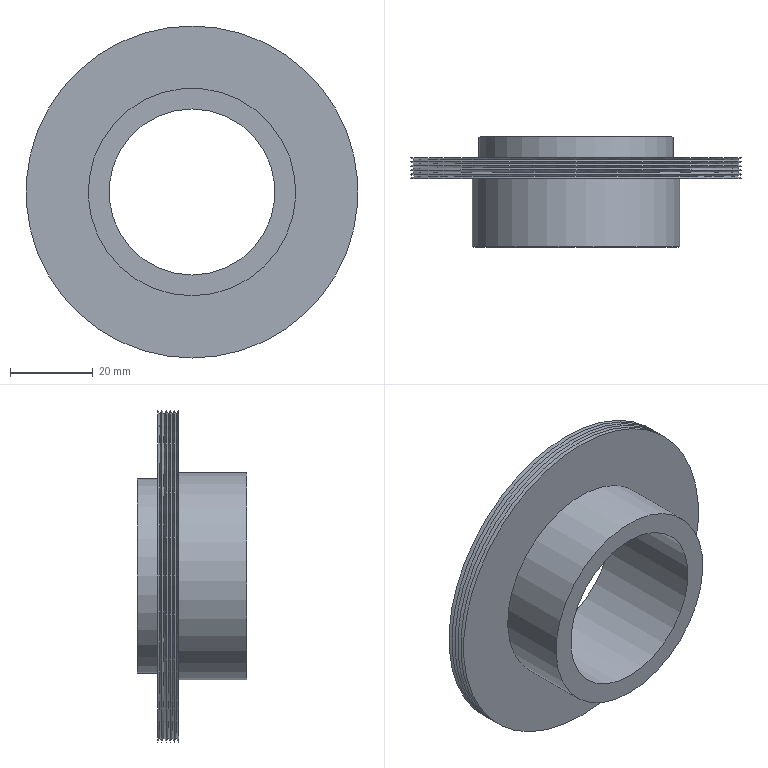Part | NX | 1 solid | 17 faces | box 80 x 26.5 x 80 mm | volume 32281 mm3 | cone 10 | plane 4 | cylinder 3 | commonest cylinder face diameters 40 x1 47 x1 50 x1
STEP:
#1=CARTESIAN_POINT('',(0.,25.732,-40.));
#2=VERTEX_POINT('',#1);
#3=CARTESIAN_POINT('',(0.,25.732,0.));
#4=DIRECTION('',(0.,-1.,0.));
#5=DIRECTION('',(0.,0.,-1.));
#6=AXIS2_PLACEMENT_3D('',#3,#4,#5);
#7=CIRCLE('',#6,40.);
#8=EDGE_CURVE('',#2,#2,#7,.T.);
#9=ORIENTED_EDGE('',*,*,#8,.F.);
#10=EDGE_LOOP('',(#9));
#11=FACE_BOUND('',#10,.T.);
#12=CARTESIAN_POINT('',(0.,25.732,-23.5));
#13=VERTEX_POINT('',#12);
#14=CARTESIAN_POINT('',(0.,25.732,0.));
#15=DIRECTION('',(0.,-1.,0.));
#16=DIRECTION('',(0.,0.,-1.));
#17=AXIS2_PLACEMENT_3D('',#14,#15,#16);
#18=CIRCLE('',#17,23.5);
#19=EDGE_CURVE('',#13,#13,#18,.T.);
#20=ORIENTED_EDGE('',*,*,#19,.T.);
#21=EDGE_LOOP('',(#20));
#22=FACE_BOUND('',#21,.T.);
#23=CARTESIAN_POINT('',(23.5,25.732,0.));
#24=DIRECTION('',(0.,-1.,0.));
#25=DIRECTION('',(0.,0.,1.));
#26=AXIS2_PLACEMENT_3D('',#23,#24,#25);
#27=PLANE('',#26);
#28=ADVANCED_FACE('',(#11,#22),#27,.F.);
#29=CARTESIAN_POINT('',(0.,25.232,-39.));
#30=VERTEX_POINT('',#29);
#31=CARTESIAN_POINT('',(0.,25.232,0.));
#32=DIRECTION('',(0.,-1.,0.));
#33=DIRECTION('',(0.,0.,-1.));
#34=AXIS2_PLACEMENT_3D('',#31,#32,#33);
#35=CIRCLE('',#34,39.);
#36=EDGE_CURVE('',#30,#30,#35,.T.);
#37=ORIENTED_EDGE('',*,*,#36,.F.);
#38=EDGE_LOOP('',(#37));
#39=FACE_BOUND('',#38,.T.);
#40=ORIENTED_EDGE('',*,*,#8,.T.);
#41=EDGE_LOOP('',(#40));
#42=FACE_BOUND('',#41,.T.);
#43=CARTESIAN_POINT('',(0.,25.732,0.));
#44=DIRECTION('',(0.,1.,0.));
#45=DIRECTION('',(0.,0.,-1.));
#46=AXIS2_PLACEMENT_3D('',#43,#44,#45);
#47=CONICAL_SURFACE('',#46,40.,63.435);
#48=ADVANCED_FACE('',(#39,#42),#47,.T.);
#49=CARTESIAN_POINT('',(0.,24.732,-40.));
#50=VERTEX_POINT('',#49);
#51=CARTESIAN_POINT('',(0.,24.732,0.));
#52=DIRECTION('',(0.,-1.,0.));
#53=DIRECTION('',(0.,0.,-1.));
#54=AXIS2_PLACEMENT_3D('',#51,#52,#53);
#55=CIRCLE('',#54,40.);
#56=EDGE_CURVE('',#50,#50,#55,.T.);
#57=ORIENTED_EDGE('',*,*,#56,.F.);
#58=EDGE_LOOP('',(#57));
#59=FACE_BOUND('',#58,.T.);
#60=ORIENTED_EDGE('',*,*,#36,.T.);
#61=EDGE_LOOP('',(#60));
#62=FACE_BOUND('',#61,.T.);
#63=CARTESIAN_POINT('',(0.,25.232,0.));
#64=DIRECTION('',(0.,-1.,0.));
#65=DIRECTION('',(0.,0.,1.));
#66=AXIS2_PLACEMENT_3D('',#63,#64,#65);
#67=CONICAL_SURFACE('',#66,39.,63.435);
#68=ADVANCED_FACE('',(#59,#62),#67,.T.);
#69=CARTESIAN_POINT('',(0.,24.232,-39.));
#70=VERTEX_POINT('',#69);
#71=CARTESIAN_POINT('',(0.,24.232,0.));
#72=DIRECTION('',(0.,-1.,0.));
#73=DIRECTION('',(0.,0.,-1.));
#74=AXIS2_PLACEMENT_3D('',#71,#72,#73);
#75=CIRCLE('',#74,39.);
#76=EDGE_CURVE('',#70,#70,#75,.T.);
#77=ORIENTED_EDGE('',*,*,#76,.F.);
#78=EDGE_LOOP('',(#77));
#79=FACE_BOUND('',#78,.T.);
#80=ORIENTED_EDGE('',*,*,#56,.T.);
#81=EDGE_LOOP('',(#80));
#82=FACE_BOUND('',#81,.T.);
#83=CARTESIAN_POINT('',(0.,24.732,0.));
#84=DIRECTION('',(0.,1.,0.));
#85=DIRECTION('',(0.,0.,-1.));
#86=AXIS2_PLACEMENT_3D('',#83,#84,#85);
#87=CONICAL_SURFACE('',#86,40.,63.435);
#88=ADVANCED_FACE('',(#79,#82),#87,.T.);
#89=CARTESIAN_POINT('',(0.,23.732,-40.));
#90=VERTEX_POINT('',#89);
#91=CARTESIAN_POINT('',(0.,23.732,0.));
#92=DIRECTION('',(0.,-1.,0.));
#93=DIRECTION('',(0.,0.,-1.));
#94=AXIS2_PLACEMENT_3D('',#91,#92,#93);
#95=CIRCLE('',#94,40.);
#96=EDGE_CURVE('',#90,#90,#95,.T.);
#97=ORIENTED_EDGE('',*,*,#96,.F.);
#98=EDGE_LOOP('',(#97));
#99=FACE_BOUND('',#98,.T.);
#100=ORIENTED_EDGE('',*,*,#76,.T.);
#101=EDGE_LOOP('',(#100));
#102=FACE_BOUND('',#101,.T.);
#103=CARTESIAN_POINT('',(0.,24.232,0.));
#104=DIRECTION('',(0.,-1.,0.));
#105=DIRECTION('',(0.,0.,1.));
#106=AXIS2_PLACEMENT_3D('',#103,#104,#105);
#107=CONICAL_SURFACE('',#106,39.,63.435);
#108=ADVANCED_FACE('',(#99,#102),#107,.T.);
#109=CARTESIAN_POINT('',(0.,23.232,-39.));
#110=VERTEX_POINT('',#109);
#111=CARTESIAN_POINT('',(0.,23.232,0.));
#112=DIRECTION('',(0.,-1.,0.));
#113=DIRECTION('',(0.,0.,-1.));
#114=AXIS2_PLACEMENT_3D('',#111,#112,#113);
#115=CIRCLE('',#114,39.);
#116=EDGE_CURVE('',#110,#110,#115,.T.);
#117=ORIENTED_EDGE('',*,*,#116,.F.);
#118=EDGE_LOOP('',(#117));
#119=FACE_BOUND('',#118,.T.);
#120=ORIENTED_EDGE('',*,*,#96,.T.);
#121=EDGE_LOOP('',(#120));
#122=FACE_BOUND('',#121,.T.);
#123=CARTESIAN_POINT('',(0.,23.732,0.));
#124=DIRECTION('',(0.,1.,0.));
#125=DIRECTION('',(0.,0.,-1.));
#126=AXIS2_PLACEMENT_3D('',#123,#124,#125);
#127=CONICAL_SURFACE('',#126,40.,63.435);
#128=ADVANCED_FACE('',(#119,#122),#127,.T.);
#129=CARTESIAN_POINT('',(0.,22.732,-40.));
#130=VERTEX_POINT('',#129);
#131=CARTESIAN_POINT('',(0.,22.732,0.));
#132=DIRECTION('',(0.,-1.,0.));
#133=DIRECTION('',(0.,0.,-1.));
#134=AXIS2_PLACEMENT_3D('',#131,#132,#133);
#135=CIRCLE('',#134,40.);
#136=EDGE_CURVE('',#130,#130,#135,.T.);
#137=ORIENTED_EDGE('',*,*,#136,.F.);
#138=EDGE_LOOP('',(#137));
#139=FACE_BOUND('',#138,.T.);
#140=ORIENTED_EDGE('',*,*,#116,.T.);
#141=EDGE_LOOP('',(#140));
#142=FACE_BOUND('',#141,.T.);
#143=CARTESIAN_POINT('',(0.,23.232,0.));
#144=DIRECTION('',(0.,-1.,0.));
#145=DIRECTION('',(0.,0.,1.));
#146=AXIS2_PLACEMENT_3D('',#143,#144,#145);
#147=CONICAL_SURFACE('',#146,39.,63.435);
#148=ADVANCED_FACE('',(#139,#142),#147,.T.);
#149=CARTESIAN_POINT('',(0.,22.232,-39.));
#150=VERTEX_POINT('',#149);
#151=CARTESIAN_POINT('',(0.,22.232,0.));
#152=DIRECTION('',(0.,-1.,0.));
#153=DIRECTION('',(0.,0.,-1.));
#154=AXIS2_PLACEMENT_3D('',#151,#152,#153);
#155=CIRCLE('',#154,39.);
#156=EDGE_CURVE('',#150,#150,#155,.T.);
#157=ORIENTED_EDGE('',*,*,#156,.F.);
#158=EDGE_LOOP('',(#157));
#159=FACE_BOUND('',#158,.T.);
#160=ORIENTED_EDGE('',*,*,#136,.T.);
#161=EDGE_LOOP('',(#160));
#162=FACE_BOUND('',#161,.T.);
#163=CARTESIAN_POINT('',(0.,22.732,0.));
#164=DIRECTION('',(0.,1.,0.));
#165=DIRECTION('',(0.,0.,-1.));
#166=AXIS2_PLACEMENT_3D('',#163,#164,#165);
#167=CONICAL_SURFACE('',#166,40.,63.435);
#168=ADVANCED_FACE('',(#159,#162),#167,.T.);
#169=CARTESIAN_POINT('',(0.,21.732,-40.));
#170=VERTEX_POINT('',#169);
#171=CARTESIAN_POINT('',(0.,21.732,0.));
#172=DIRECTION('',(0.,-1.,0.));
#173=DIRECTION('',(0.,0.,-1.));
#174=AXIS2_PLACEMENT_3D('',#171,#172,#173);
#175=CIRCLE('',#174,40.);
#176=EDGE_CURVE('',#170,#170,#175,.T.);
#177=ORIENTED_EDGE('',*,*,#176,.F.);
#178=EDGE_LOOP('',(#177));
#179=FACE_BOUND('',#178,.T.);
#180=ORIENTED_EDGE('',*,*,#156,.T.);
#181=EDGE_LOOP('',(#180));
#182=FACE_BOUND('',#181,.T.);
#183=CARTESIAN_POINT('',(0.,22.232,0.));
#184=DIRECTION('',(0.,-1.,0.));
#185=DIRECTION('',(0.,0.,1.));
#186=AXIS2_PLACEMENT_3D('',#183,#184,#185);
#187=CONICAL_SURFACE('',#186,39.,63.435);
#188=ADVANCED_FACE('',(#179,#182),#187,.T.);
#189=CARTESIAN_POINT('',(0.,21.232,-39.));
#190=VERTEX_POINT('',#189);
#191=CARTESIAN_POINT('',(0.,21.232,0.));
#192=DIRECTION('',(0.,-1.,0.));
#193=DIRECTION('',(0.,0.,-1.));
#194=AXIS2_PLACEMENT_3D('',#191,#192,#193);
#195=CIRCLE('',#194,39.);
#196=EDGE_CURVE('',#190,#190,#195,.T.);
#197=ORIENTED_EDGE('',*,*,#196,.F.);
#198=EDGE_LOOP('',(#197));
#199=FACE_BOUND('',#198,.T.);
#200=ORIENTED_EDGE('',*,*,#176,.T.);
#201=EDGE_LOOP('',(#200));
#202=FACE_BOUND('',#201,.T.);
#203=CARTESIAN_POINT('',(0.,21.732,0.));
#204=DIRECTION('',(0.,1.,0.));
#205=DIRECTION('',(0.,0.,-1.));
#206=AXIS2_PLACEMENT_3D('',#203,#204,#205);
#207=CONICAL_SURFACE('',#206,40.,63.435);
#208=ADVANCED_FACE('',(#199,#202),#207,.T.);
#209=CARTESIAN_POINT('',(0.,20.732,-40.));
#210=VERTEX_POINT('',#209);
#211=CARTESIAN_POINT('',(0.,20.732,0.));
#212=DIRECTION('',(0.,-1.,0.));
#213=DIRECTION('',(0.,0.,-1.));
#214=AXIS2_PLACEMENT_3D('',#211,#212,#213);
#215=CIRCLE('',#214,40.);
#216=EDGE_CURVE('',#210,#210,#215,.T.);
#217=ORIENTED_EDGE('',*,*,#216,.F.);
#218=EDGE_LOOP('',(#217));
#219=FACE_BOUND('',#218,.T.);
#220=ORIENTED_EDGE('',*,*,#196,.T.);
#221=EDGE_LOOP('',(#220));
#222=FACE_BOUND('',#221,.T.);
#223=CARTESIAN_POINT('',(0.,21.232,0.));
#224=DIRECTION('',(0.,-1.,0.));
#225=DIRECTION('',(0.,0.,1.));
#226=AXIS2_PLACEMENT_3D('',#223,#224,#225);
#227=CONICAL_SURFACE('',#226,39.,63.435);
#228=ADVANCED_FACE('',(#219,#222),#227,.T.);
#229=CARTESIAN_POINT('',(0.,20.732,-25.));
#230=VERTEX_POINT('',#229);
#231=CARTESIAN_POINT('',(0.,20.732,0.));
#232=DIRECTION('',(0.,-1.,0.));
#233=DIRECTION('',(0.,0.,-1.));
#234=AXIS2_PLACEMENT_3D('',#231,#232,#233);
#235=CIRCLE('',#234,25.);
#236=EDGE_CURVE('',#230,#230,#235,.T.);
#237=ORIENTED_EDGE('',*,*,#236,.F.);
#238=EDGE_LOOP('',(#237));
#239=FACE_BOUND('',#238,.T.);
#240=ORIENTED_EDGE('',*,*,#216,.T.);
#241=EDGE_LOOP('',(#240));
#242=FACE_BOUND('',#241,.T.);
#243=CARTESIAN_POINT('',(40.,20.732,0.));
#244=DIRECTION('',(0.,1.,0.));
#245=DIRECTION('',(0.,0.,-1.));
#246=AXIS2_PLACEMENT_3D('',#243,#244,#245);
#247=PLANE('',#246);
#248=ADVANCED_FACE('',(#239,#242),#247,.F.);
#249=CARTESIAN_POINT('',(0.,4.232,-25.));
#250=VERTEX_POINT('',#249);
#251=CARTESIAN_POINT('',(0.,4.232,0.));
#252=DIRECTION('',(0.,-1.,0.));
#253=DIRECTION('',(0.,0.,-1.));
#254=AXIS2_PLACEMENT_3D('',#251,#252,#253);
#255=CIRCLE('',#254,25.);
#256=EDGE_CURVE('',#250,#250,#255,.T.);
#257=ORIENTED_EDGE('',*,*,#256,.F.);
#258=EDGE_LOOP('',(#257));
#259=FACE_BOUND('',#258,.T.);
#260=ORIENTED_EDGE('',*,*,#236,.T.);
#261=EDGE_LOOP('',(#260));
#262=FACE_BOUND('',#261,.T.);
#263=CARTESIAN_POINT('',(0.,35.105,0.));
#264=DIRECTION('',(0.,-1.,0.));
#265=DIRECTION('',(0.,0.,1.));
#266=AXIS2_PLACEMENT_3D('',#263,#264,#265);
#267=CYLINDRICAL_SURFACE('',#266,25.);
#268=ADVANCED_FACE('',(#259,#262),#267,.T.);
#269=CARTESIAN_POINT('',(0.,4.232,-20.));
#270=VERTEX_POINT('',#269);
#271=CARTESIAN_POINT('',(0.,4.232,0.));
#272=DIRECTION('',(0.,-1.,0.));
#273=DIRECTION('',(0.,0.,-1.));
#274=AXIS2_PLACEMENT_3D('',#271,#272,#273);
#275=CIRCLE('',#274,20.);
#276=EDGE_CURVE('',#270,#270,#275,.T.);
#277=ORIENTED_EDGE('',*,*,#276,.F.);
#278=EDGE_LOOP('',(#277));
#279=FACE_BOUND('',#278,.T.);
#280=ORIENTED_EDGE('',*,*,#256,.T.);
#281=EDGE_LOOP('',(#280));
#282=FACE_BOUND('',#281,.T.);
#283=CARTESIAN_POINT('',(25.,4.232,0.));
#284=DIRECTION('',(0.,1.,0.));
#285=DIRECTION('',(0.,0.,-1.));
#286=AXIS2_PLACEMENT_3D('',#283,#284,#285);
#287=PLANE('',#286);
#288=ADVANCED_FACE('',(#279,#282),#287,.F.);
#289=CARTESIAN_POINT('',(0.,30.732,-20.));
#290=VERTEX_POINT('',#289);
#291=CARTESIAN_POINT('',(0.,30.732,0.));
#292=DIRECTION('',(0.,-1.,0.));
#293=DIRECTION('',(0.,0.,-1.));
#294=AXIS2_PLACEMENT_3D('',#291,#292,#293);
#295=CIRCLE('',#294,20.);
#296=EDGE_CURVE('',#290,#290,#295,.T.);
#297=ORIENTED_EDGE('',*,*,#296,.F.);
#298=EDGE_LOOP('',(#297));
#299=FACE_BOUND('',#298,.T.);
#300=ORIENTED_EDGE('',*,*,#276,.T.);
#301=EDGE_LOOP('',(#300));
#302=FACE_BOUND('',#301,.T.);
#303=CARTESIAN_POINT('',(0.,35.105,0.));
#304=DIRECTION('',(0.,-1.,0.));
#305=DIRECTION('',(0.,0.,1.));
#306=AXIS2_PLACEMENT_3D('',#303,#304,#305);
#307=CYLINDRICAL_SURFACE('',#306,20.);
#308=ADVANCED_FACE('',(#299,#302),#307,.F.);
#309=CARTESIAN_POINT('',(0.,30.732,-23.5));
#310=VERTEX_POINT('',#309);
#311=CARTESIAN_POINT('',(0.,30.732,0.));
#312=DIRECTION('',(0.,-1.,0.));
#313=DIRECTION('',(0.,0.,-1.));
#314=AXIS2_PLACEMENT_3D('',#311,#312,#313);
#315=CIRCLE('',#314,23.5);
#316=EDGE_CURVE('',#310,#310,#315,.T.);
#317=ORIENTED_EDGE('',*,*,#316,.F.);
#318=EDGE_LOOP('',(#317));
#319=FACE_BOUND('',#318,.T.);
#320=ORIENTED_EDGE('',*,*,#296,.T.);
#321=EDGE_LOOP('',(#320));
#322=FACE_BOUND('',#321,.T.);
#323=CARTESIAN_POINT('',(20.,30.732,0.));
#324=DIRECTION('',(0.,-1.,0.));
#325=DIRECTION('',(0.,0.,1.));
#326=AXIS2_PLACEMENT_3D('',#323,#324,#325);
#327=PLANE('',#326);
#328=ADVANCED_FACE('',(#319,#322),#327,.F.);
#329=ORIENTED_EDGE('',*,*,#19,.F.);
#330=EDGE_LOOP('',(#329));
#331=FACE_BOUND('',#330,.T.);
#332=ORIENTED_EDGE('',*,*,#316,.T.);
#333=EDGE_LOOP('',(#332));
#334=FACE_BOUND('',#333,.T.);
#335=CARTESIAN_POINT('',(0.,35.105,0.));
#336=DIRECTION('',(0.,-1.,0.));
#337=DIRECTION('',(0.,0.,1.));
#338=AXIS2_PLACEMENT_3D('',#335,#336,#337);
#339=CYLINDRICAL_SURFACE('',#338,23.5);
#340=ADVANCED_FACE('',(#331,#334),#339,.T.);
#341=CLOSED_SHELL('',(#28,#48,#68,#88,#108,#128,#148,#168,#188,#208,#228,#248,#268,#288,#308,#328,#340));
#342=MANIFOLD_SOLID_BREP('',#341);
#343=(LENGTH_UNIT()NAMED_UNIT(*)SI_UNIT(.MILLI.,.METRE.));
#344=UNCERTAINTY_MEASURE_WITH_UNIT(LENGTH_MEASURE(0.00002),#343,'','');
#345=(NAMED_UNIT(*)PLANE_ANGLE_UNIT()SI_UNIT($,.RADIAN.));
#346=PLANE_ANGLE_MEASURE_WITH_UNIT(PLANE_ANGLE_MEASURE(0.01745),#345);
#347=DIMENSIONAL_EXPONENTS(0.,0.,0.,0.,0.,0.,0.);
#348=(CONVERSION_BASED_UNIT('DEGREE',#346)NAMED_UNIT(#347)PLANE_ANGLE_UNIT());
#349=(NAMED_UNIT(*)SI_UNIT($,.STERADIAN.)SOLID_ANGLE_UNIT());
#350=(GEOMETRIC_REPRESENTATION_CONTEXT(3)GLOBAL_UNCERTAINTY_ASSIGNED_CONTEXT((#344))GLOBAL_UNIT_ASSIGNED_CONTEXT((#343,#348,#349))REPRESENTATION_CONTEXT('',''));
#351=ADVANCED_BREP_SHAPE_REPRESENTATION('',(#342),#350);